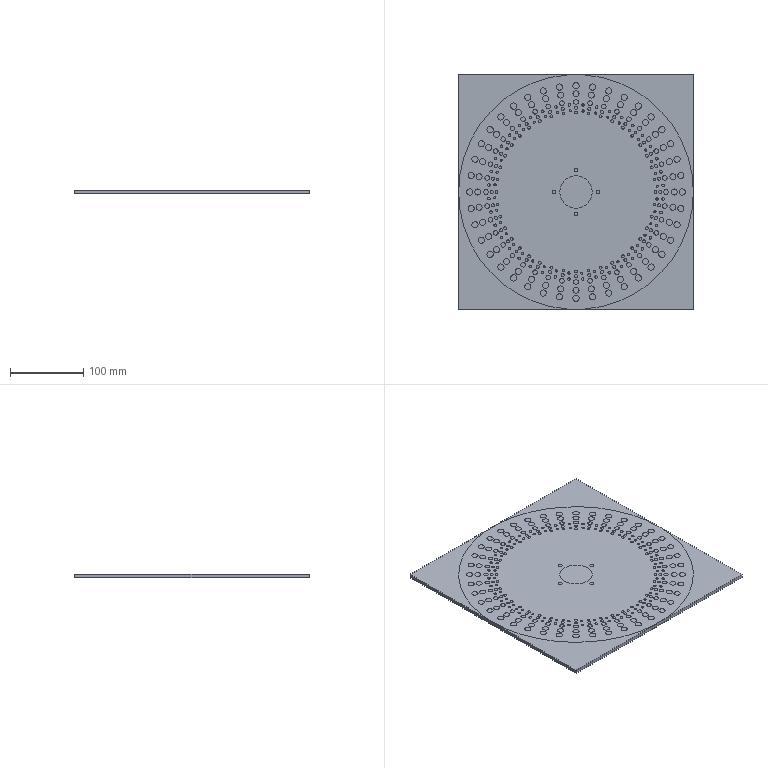CAM job | NX | 3-axis milling, drilling | part box 320 x 320 x 5 mm | stock box 320 x 320 x 5 mm
Tools:
number,name,description,diameter,corner_radius,flute_length,length,flutes
0,D6点孔钻,Drilling Tool,10.0,0.0,5.0,40.0,2
0,D17R0.8圆鼻飞刀,Milling Tool-5 Parameters,17.0,0.8,60.0,60.0,2
8,D6平底刀,Milling Tool-5 Parameters,4.5,0.0,15.0,20.0,3
Operations:
program,operation,operation_type,tool,method,geometry_group,spindle_rpm,surface_speed,feed_per_tooth,feed_cut,feed_plunge,cut_length_mm,path_length_mm,cut_time_min,machine_time_min
1,等高外形,ZLevelMilling,D17R0.8圆鼻飞刀,METHOD,WORKPIECE---A,2000.0,106.0,0.5,2000.0,80.0,57188.256,57232.856,28.595,28.6
1,G81点孔,Operation,D6点孔钻,METHOD,WORKPIECE---A,1500.0,47.0,0.02,60.0,0.0,855.0,5369.865,14.25,14.701
1.NC_1,孔铣精光G41,CylinderMilling,D6平底刀,METHOD,WORKPIECE---A,3000.0,42.0,0.0556,500.0,80.0,14044.835,16674.658,28.173,28.436
1.NC_1,孔铣精光G41_COPY,CylinderMilling,D6平底刀,METHOD,WORKPIECE---A,3000.0,42.0,0.0556,500.0,80.0,13008.195,15591.563,26.095,26.354
1.NC,等高外形_COPY,ZLevelMilling,D17R0.8圆鼻飞刀,METHOD,WORKPIECE---A,2000.0,106.0,0.5,2000.0,80.0,2915.762,2960.361,1.458,1.463
1.NC,等高外形_COPY_1,ZLevelMilling,D17R0.8圆鼻飞刀,METHOD,WORKPIECE---A,2000.0,106.0,0.5,2000.0,80.0,4621.658,4666.257,2.312,2.316
1.NC,孔铣精光G41_1,CylinderMilling,D17R0.8圆鼻飞刀,METHOD,MCS---A,2000.0,106.0,0.125,500.0,80.0,2346.795,2390.395,4.705,4.709